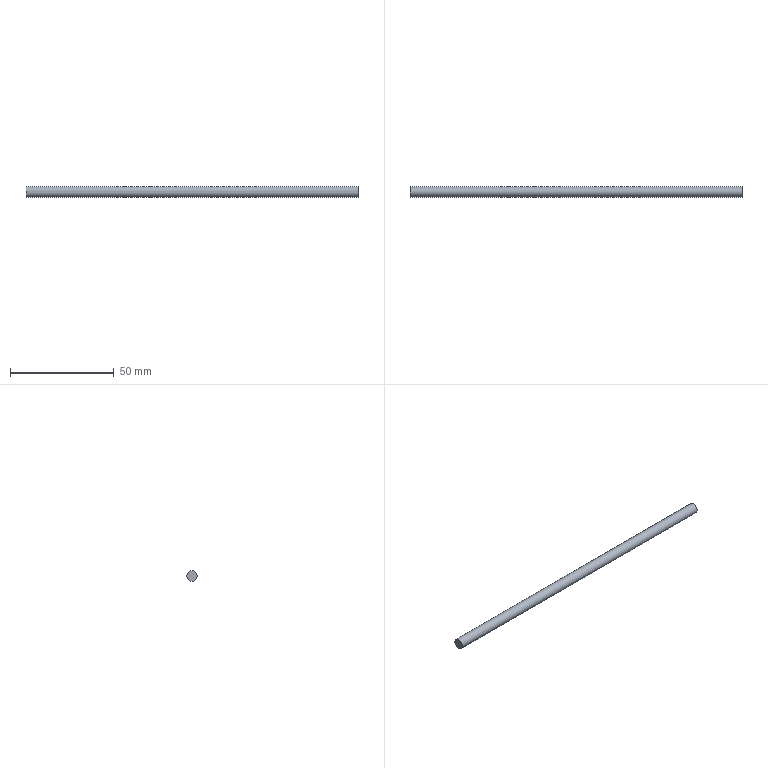Part | NX | features solid 2 | 1 solid | 3 faces | box 160 x 5 x 5 mm | volume 3142 mm3 | plane 2 | cylinder 1 | commonest cylinder face diameters 5 x1
STEP:
#1=CARTESIAN_POINT('',(262.,377.5,-372.5));
#2=VERTEX_POINT('',#1);
#3=CARTESIAN_POINT('',(262.,377.5,-375.));
#4=DIRECTION('',(-1.,0.,0.));
#5=DIRECTION('',(0.,0.,1.));
#6=AXIS2_PLACEMENT_3D('',#3,#4,#5);
#7=CIRCLE('',#6,2.5);
#8=EDGE_CURVE('',#2,#2,#7,.T.);
#9=ORIENTED_EDGE('',*,*,#8,.F.);
#10=EDGE_LOOP('',(#9));
#11=FACE_BOUND('',#10,.T.);
#12=CARTESIAN_POINT('',(422.,377.5,-372.5));
#13=VERTEX_POINT('',#12);
#14=CARTESIAN_POINT('',(422.,377.5,-375.));
#15=DIRECTION('',(-1.,0.,0.));
#16=DIRECTION('',(0.,0.,1.));
#17=AXIS2_PLACEMENT_3D('',#14,#15,#16);
#18=CIRCLE('',#17,2.5);
#19=EDGE_CURVE('',#13,#13,#18,.T.);
#20=ORIENTED_EDGE('',*,*,#19,.T.);
#21=EDGE_LOOP('',(#20));
#22=FACE_BOUND('',#21,.T.);
#23=CARTESIAN_POINT('',(262.,377.5,-375.));
#24=DIRECTION('',(1.,0.,0.));
#25=DIRECTION('',(0.,0.,-1.));
#26=AXIS2_PLACEMENT_3D('',#23,#24,#25);
#27=CYLINDRICAL_SURFACE('',#26,2.5);
#28=ADVANCED_FACE('',(#11,#22),#27,.T.);
#29=ORIENTED_EDGE('',*,*,#8,.T.);
#30=EDGE_LOOP('',(#29));
#31=FACE_BOUND('',#30,.T.);
#32=CARTESIAN_POINT('',(262.,377.5,-375.));
#33=DIRECTION('',(-1.,0.,0.));
#34=DIRECTION('',(0.,0.,1.));
#35=AXIS2_PLACEMENT_3D('',#32,#33,#34);
#36=PLANE('',#35);
#37=ADVANCED_FACE('',(#31),#36,.T.);
#38=ORIENTED_EDGE('',*,*,#19,.F.);
#39=EDGE_LOOP('',(#38));
#40=FACE_BOUND('',#39,.T.);
#41=CARTESIAN_POINT('',(422.,377.5,-375.));
#42=DIRECTION('',(-1.,0.,0.));
#43=DIRECTION('',(0.,0.,1.));
#44=AXIS2_PLACEMENT_3D('',#41,#42,#43);
#45=PLANE('',#44);
#46=ADVANCED_FACE('',(#40),#45,.F.);
#47=CLOSED_SHELL('',(#28,#37,#46));
#48=MANIFOLD_SOLID_BREP('',#47);
#49=(LENGTH_UNIT()NAMED_UNIT(*)SI_UNIT(.MILLI.,.METRE.));
#50=UNCERTAINTY_MEASURE_WITH_UNIT(LENGTH_MEASURE(0.00001),#49,'','');
#51=(NAMED_UNIT(*)PLANE_ANGLE_UNIT()SI_UNIT($,.RADIAN.));
#52=(NAMED_UNIT(*)SI_UNIT($,.STERADIAN.)SOLID_ANGLE_UNIT());
#53=(GEOMETRIC_REPRESENTATION_CONTEXT(3)GLOBAL_UNCERTAINTY_ASSIGNED_CONTEXT((#50))GLOBAL_UNIT_ASSIGNED_CONTEXT((#49,#51,#52))REPRESENTATION_CONTEXT('',''));
#54=ADVANCED_BREP_SHAPE_REPRESENTATION('',(#48),#53);